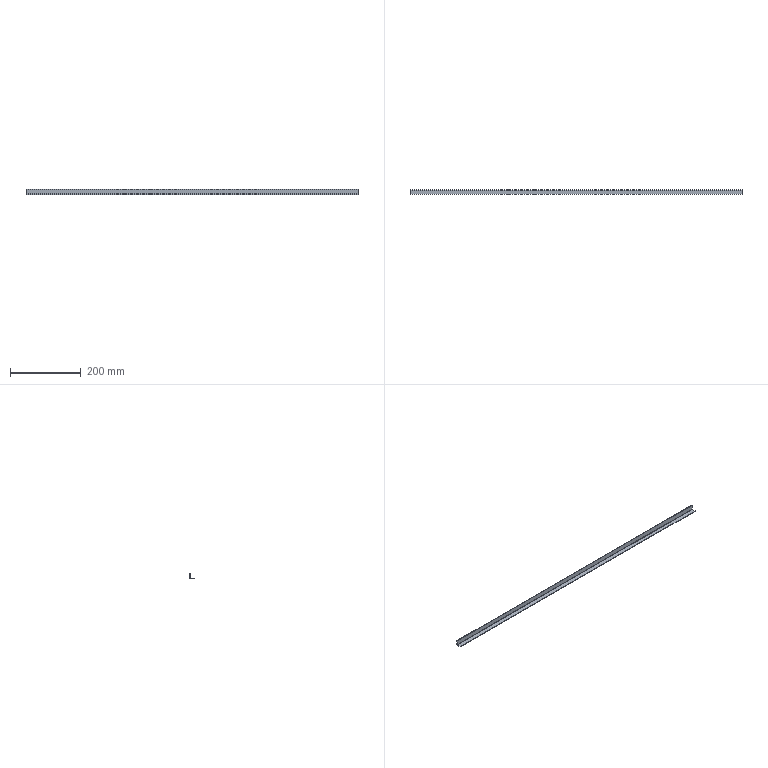Part | STEP file | Left Side Panel Frame Lower | 1 solid | 10 faces | box 940 x 13.5 x 15 mm | volume 37314 mm3 | plane 8 | cylinder 2 | commonest cylinder face diameters 1 x1 4 x1
STEP:
#1=CARTESIAN_POINT('',(940.,0.,0.));
#2=VERTEX_POINT('',#1);
#3=CARTESIAN_POINT('',(940.,0.,-13.));
#4=VERTEX_POINT('',#3);
#5=CARTESIAN_POINT('',(940.,0.,0.));
#6=DIRECTION('',(0.,0.,-1.));
#7=VECTOR('',#6,1000.);
#8=LINE('',#5,#7);
#9=EDGE_CURVE('',#2,#4,#8,.T.);
#10=ORIENTED_EDGE('',*,*,#9,.T.);
#11=CARTESIAN_POINT('',(0.,0.,-13.));
#12=VERTEX_POINT('',#11);
#13=CARTESIAN_POINT('',(940.,0.,-13.));
#14=DIRECTION('',(-1.,0.,0.));
#15=VECTOR('',#14,1000.);
#16=LINE('',#13,#15);
#17=EDGE_CURVE('',#4,#12,#16,.T.);
#18=ORIENTED_EDGE('',*,*,#17,.T.);
#19=CARTESIAN_POINT('',(0.,0.,0.));
#20=VERTEX_POINT('',#19);
#21=CARTESIAN_POINT('',(0.,0.,0.));
#22=DIRECTION('',(0.,0.,1.));
#23=VECTOR('',#22,1000.);
#24=LINE('',#21,#23);
#25=EDGE_CURVE('',#12,#20,#24,.T.);
#26=ORIENTED_EDGE('',*,*,#25,.T.);
#27=CARTESIAN_POINT('',(940.,0.,0.));
#28=DIRECTION('',(1.,0.,0.));
#29=VECTOR('',#28,1000.);
#30=LINE('',#27,#29);
#31=EDGE_CURVE('',#20,#2,#30,.T.);
#32=ORIENTED_EDGE('',*,*,#31,.T.);
#33=EDGE_LOOP('',(#10,#18,#26,#32));
#34=FACE_OUTER_BOUND('',#33,.T.);
#35=CARTESIAN_POINT('',(940.,0.,0.));
#36=DIRECTION('',(0.,1.,0.));
#37=DIRECTION('',(0.,0.,1.));
#38=AXIS2_PLACEMENT_3D('',#35,#36,#37);
#39=PLANE('',#38);
#40=ADVANCED_FACE('',(#34),#39,.T.);
#41=CARTESIAN_POINT('',(940.,-2.,-15.));
#42=VERTEX_POINT('',#41);
#43=CARTESIAN_POINT('',(940.,-2.,-13.));
#44=DIRECTION('',(-1.,0.,0.));
#45=DIRECTION('',(0.,0.,1.));
#46=AXIS2_PLACEMENT_3D('',#43,#44,#45);
#47=CIRCLE('',#46,2.);
#48=EDGE_CURVE('',#4,#42,#47,.T.);
#49=ORIENTED_EDGE('',*,*,#48,.T.);
#50=CARTESIAN_POINT('',(0.,-2.,-15.));
#51=VERTEX_POINT('',#50);
#52=CARTESIAN_POINT('',(940.,-2.,-15.));
#53=DIRECTION('',(-1.,0.,0.));
#54=VECTOR('',#53,1000.);
#55=LINE('',#52,#54);
#56=EDGE_CURVE('',#42,#51,#55,.T.);
#57=ORIENTED_EDGE('',*,*,#56,.T.);
#58=CARTESIAN_POINT('',(0.,-2.,-13.));
#59=DIRECTION('',(1.,0.,0.));
#60=DIRECTION('',(0.,0.,1.));
#61=AXIS2_PLACEMENT_3D('',#58,#59,#60);
#62=CIRCLE('',#61,2.);
#63=EDGE_CURVE('',#51,#12,#62,.T.);
#64=ORIENTED_EDGE('',*,*,#63,.T.);
#65=ORIENTED_EDGE('',*,*,#17,.F.);
#66=EDGE_LOOP('',(#49,#57,#64,#65));
#67=FACE_OUTER_BOUND('',#66,.T.);
#68=CARTESIAN_POINT('',(940.,-2.,-13.));
#69=DIRECTION('',(-1.,0.,0.));
#70=DIRECTION('',(0.,0.,1.));
#71=AXIS2_PLACEMENT_3D('',#68,#69,#70);
#72=CYLINDRICAL_SURFACE('',#71,2.);
#73=ADVANCED_FACE('',(#67),#72,.T.);
#74=ORIENTED_EDGE('',*,*,#9,.F.);
#75=CARTESIAN_POINT('',(940.,-1.5,0.));
#76=VERTEX_POINT('',#75);
#77=CARTESIAN_POINT('',(940.,-2.,0.));
#78=DIRECTION('',(0.,-1.,0.));
#79=VECTOR('',#78,1000.);
#80=LINE('',#77,#79);
#81=EDGE_CURVE('',#2,#76,#80,.T.);
#82=ORIENTED_EDGE('',*,*,#81,.T.);
#83=CARTESIAN_POINT('',(940.,-1.5,-13.));
#84=VERTEX_POINT('',#83);
#85=CARTESIAN_POINT('',(940.,-1.5,-13.));
#86=DIRECTION('',(0.,0.,-1.));
#87=VECTOR('',#86,1000.);
#88=LINE('',#85,#87);
#89=EDGE_CURVE('',#76,#84,#88,.T.);
#90=ORIENTED_EDGE('',*,*,#89,.T.);
#91=CARTESIAN_POINT('',(940.,-2.,-13.5));
#92=VERTEX_POINT('',#91);
#93=CARTESIAN_POINT('',(940.,-2.,-13.));
#94=DIRECTION('',(-1.,0.,0.));
#95=DIRECTION('',(0.,0.,1.));
#96=AXIS2_PLACEMENT_3D('',#93,#94,#95);
#97=CIRCLE('',#96,0.5);
#98=EDGE_CURVE('',#84,#92,#97,.T.);
#99=ORIENTED_EDGE('',*,*,#98,.T.);
#100=CARTESIAN_POINT('',(940.,-13.5,-13.5));
#101=VERTEX_POINT('',#100);
#102=CARTESIAN_POINT('',(940.,-1.5,-13.5));
#103=DIRECTION('',(0.,-1.,0.));
#104=VECTOR('',#103,1000.);
#105=LINE('',#102,#104);
#106=EDGE_CURVE('',#92,#101,#105,.T.);
#107=ORIENTED_EDGE('',*,*,#106,.T.);
#108=CARTESIAN_POINT('',(940.,-13.5,-15.));
#109=VERTEX_POINT('',#108);
#110=CARTESIAN_POINT('',(940.,-13.5,-15.));
#111=DIRECTION('',(0.,0.,1.));
#112=VECTOR('',#111,1000.);
#113=LINE('',#110,#112);
#114=EDGE_CURVE('',#109,#101,#113,.T.);
#115=ORIENTED_EDGE('',*,*,#114,.F.);
#116=CARTESIAN_POINT('',(940.,0.,-15.));
#117=DIRECTION('',(0.,-1.,0.));
#118=VECTOR('',#117,1000.);
#119=LINE('',#116,#118);
#120=EDGE_CURVE('',#42,#109,#119,.T.);
#121=ORIENTED_EDGE('',*,*,#120,.F.);
#122=ORIENTED_EDGE('',*,*,#48,.F.);
#123=EDGE_LOOP('',(#74,#82,#90,#99,#107,#115,#121,#122));
#124=FACE_OUTER_BOUND('',#123,.T.);
#125=CARTESIAN_POINT('',(940.,-2.,-13.));
#126=DIRECTION('',(1.,0.,0.));
#127=DIRECTION('',(0.,0.,-1.));
#128=AXIS2_PLACEMENT_3D('',#125,#126,#127);
#129=PLANE('',#128);
#130=ADVANCED_FACE('',(#124),#129,.T.);
#131=ORIENTED_EDGE('',*,*,#81,.F.);
#132=ORIENTED_EDGE('',*,*,#31,.F.);
#133=CARTESIAN_POINT('',(0.,-1.5,0.));
#134=VERTEX_POINT('',#133);
#135=CARTESIAN_POINT('',(0.,-1.5,0.));
#136=DIRECTION('',(0.,-1.,0.));
#137=VECTOR('',#136,1000.);
#138=LINE('',#135,#137);
#139=EDGE_CURVE('',#20,#134,#138,.T.);
#140=ORIENTED_EDGE('',*,*,#139,.T.);
#141=CARTESIAN_POINT('',(940.,-1.5,0.));
#142=DIRECTION('',(1.,0.,0.));
#143=VECTOR('',#142,1000.);
#144=LINE('',#141,#143);
#145=EDGE_CURVE('',#134,#76,#144,.T.);
#146=ORIENTED_EDGE('',*,*,#145,.T.);
#147=EDGE_LOOP('',(#131,#132,#140,#146));
#148=FACE_OUTER_BOUND('',#147,.T.);
#149=CARTESIAN_POINT('',(940.,-1.5,0.));
#150=DIRECTION('',(0.,0.,1.));
#151=DIRECTION('',(1.,0.,0.));
#152=AXIS2_PLACEMENT_3D('',#149,#150,#151);
#153=PLANE('',#152);
#154=ADVANCED_FACE('',(#148),#153,.T.);
#155=CARTESIAN_POINT('',(0.,-1.5,-13.));
#156=VERTEX_POINT('',#155);
#157=CARTESIAN_POINT('',(0.,-1.5,-13.5));
#158=DIRECTION('',(0.,0.,1.));
#159=VECTOR('',#158,1000.);
#160=LINE('',#157,#159);
#161=EDGE_CURVE('',#156,#134,#160,.T.);
#162=ORIENTED_EDGE('',*,*,#161,.T.);
#163=ORIENTED_EDGE('',*,*,#139,.F.);
#164=ORIENTED_EDGE('',*,*,#25,.F.);
#165=ORIENTED_EDGE('',*,*,#63,.F.);
#166=CARTESIAN_POINT('',(0.,-13.5,-15.));
#167=VERTEX_POINT('',#166);
#168=CARTESIAN_POINT('',(0.,0.,-15.));
#169=DIRECTION('',(0.,1.,0.));
#170=VECTOR('',#169,1000.);
#171=LINE('',#168,#170);
#172=EDGE_CURVE('',#167,#51,#171,.T.);
#173=ORIENTED_EDGE('',*,*,#172,.F.);
#174=CARTESIAN_POINT('',(0.,-13.5,-13.5));
#175=VERTEX_POINT('',#174);
#176=CARTESIAN_POINT('',(0.,-13.5,-15.));
#177=DIRECTION('',(0.,0.,-1.));
#178=VECTOR('',#177,1000.);
#179=LINE('',#176,#178);
#180=EDGE_CURVE('',#175,#167,#179,.T.);
#181=ORIENTED_EDGE('',*,*,#180,.F.);
#182=CARTESIAN_POINT('',(0.,-2.,-13.5));
#183=VERTEX_POINT('',#182);
#184=CARTESIAN_POINT('',(0.,-2.,-13.5));
#185=DIRECTION('',(0.,-1.,0.));
#186=VECTOR('',#185,1000.);
#187=LINE('',#184,#186);
#188=EDGE_CURVE('',#183,#175,#187,.T.);
#189=ORIENTED_EDGE('',*,*,#188,.F.);
#190=CARTESIAN_POINT('',(0.,-2.,-13.));
#191=DIRECTION('',(1.,0.,0.));
#192=DIRECTION('',(0.,0.,1.));
#193=AXIS2_PLACEMENT_3D('',#190,#191,#192);
#194=CIRCLE('',#193,0.5);
#195=EDGE_CURVE('',#183,#156,#194,.T.);
#196=ORIENTED_EDGE('',*,*,#195,.T.);
#197=EDGE_LOOP('',(#162,#163,#164,#165,#173,#181,#189,#196));
#198=FACE_OUTER_BOUND('',#197,.T.);
#199=CARTESIAN_POINT('',(0.,-2.,-13.5));
#200=DIRECTION('',(-1.,0.,0.));
#201=DIRECTION('',(0.,0.,1.));
#202=AXIS2_PLACEMENT_3D('',#199,#200,#201);
#203=PLANE('',#202);
#204=ADVANCED_FACE('',(#198),#203,.T.);
#205=ORIENTED_EDGE('',*,*,#120,.T.);
#206=CARTESIAN_POINT('',(940.,-13.5,-15.));
#207=DIRECTION('',(-1.,0.,0.));
#208=VECTOR('',#207,1000.);
#209=LINE('',#206,#208);
#210=EDGE_CURVE('',#109,#167,#209,.T.);
#211=ORIENTED_EDGE('',*,*,#210,.T.);
#212=ORIENTED_EDGE('',*,*,#172,.T.);
#213=ORIENTED_EDGE('',*,*,#56,.F.);
#214=EDGE_LOOP('',(#205,#211,#212,#213));
#215=FACE_OUTER_BOUND('',#214,.T.);
#216=CARTESIAN_POINT('',(940.,0.,-15.));
#217=DIRECTION('',(0.,0.,-1.));
#218=DIRECTION('',(0.,1.,0.));
#219=AXIS2_PLACEMENT_3D('',#216,#217,#218);
#220=PLANE('',#219);
#221=ADVANCED_FACE('',(#215),#220,.T.);
#222=CARTESIAN_POINT('',(940.,-1.5,-13.));
#223=DIRECTION('',(-1.,0.,0.));
#224=VECTOR('',#223,1000.);
#225=LINE('',#222,#224);
#226=EDGE_CURVE('',#84,#156,#225,.T.);
#227=ORIENTED_EDGE('',*,*,#226,.F.);
#228=ORIENTED_EDGE('',*,*,#89,.F.);
#229=ORIENTED_EDGE('',*,*,#145,.F.);
#230=ORIENTED_EDGE('',*,*,#161,.F.);
#231=EDGE_LOOP('',(#227,#228,#229,#230));
#232=FACE_OUTER_BOUND('',#231,.T.);
#233=CARTESIAN_POINT('',(940.,-1.5,0.));
#234=DIRECTION('',(0.,1.,0.));
#235=DIRECTION('',(0.,0.,1.));
#236=AXIS2_PLACEMENT_3D('',#233,#234,#235);
#237=PLANE('',#236);
#238=ADVANCED_FACE('',(#232),#237,.F.);
#239=ORIENTED_EDGE('',*,*,#114,.T.);
#240=CARTESIAN_POINT('',(940.,-13.5,-13.5));
#241=DIRECTION('',(-1.,0.,0.));
#242=VECTOR('',#241,1000.);
#243=LINE('',#240,#242);
#244=EDGE_CURVE('',#101,#175,#243,.T.);
#245=ORIENTED_EDGE('',*,*,#244,.T.);
#246=ORIENTED_EDGE('',*,*,#180,.T.);
#247=ORIENTED_EDGE('',*,*,#210,.F.);
#248=EDGE_LOOP('',(#239,#245,#246,#247));
#249=FACE_OUTER_BOUND('',#248,.T.);
#250=CARTESIAN_POINT('',(940.,-13.5,-15.));
#251=DIRECTION('',(0.,-1.,0.));
#252=DIRECTION('',(0.,0.,-1.));
#253=AXIS2_PLACEMENT_3D('',#250,#251,#252);
#254=PLANE('',#253);
#255=ADVANCED_FACE('',(#249),#254,.T.);
#256=CARTESIAN_POINT('',(940.,-2.,-13.5));
#257=DIRECTION('',(-1.,0.,0.));
#258=VECTOR('',#257,1000.);
#259=LINE('',#256,#258);
#260=EDGE_CURVE('',#92,#183,#259,.T.);
#261=ORIENTED_EDGE('',*,*,#260,.F.);
#262=ORIENTED_EDGE('',*,*,#98,.F.);
#263=ORIENTED_EDGE('',*,*,#226,.T.);
#264=ORIENTED_EDGE('',*,*,#195,.F.);
#265=EDGE_LOOP('',(#261,#262,#263,#264));
#266=FACE_OUTER_BOUND('',#265,.T.);
#267=CARTESIAN_POINT('',(940.,-2.,-13.));
#268=DIRECTION('',(-1.,0.,0.));
#269=DIRECTION('',(0.,0.,1.));
#270=AXIS2_PLACEMENT_3D('',#267,#268,#269);
#271=CYLINDRICAL_SURFACE('',#270,0.5);
#272=ADVANCED_FACE('',(#266),#271,.F.);
#273=ORIENTED_EDGE('',*,*,#244,.F.);
#274=ORIENTED_EDGE('',*,*,#106,.F.);
#275=ORIENTED_EDGE('',*,*,#260,.T.);
#276=ORIENTED_EDGE('',*,*,#188,.T.);
#277=EDGE_LOOP('',(#273,#274,#275,#276));
#278=FACE_OUTER_BOUND('',#277,.T.);
#279=CARTESIAN_POINT('',(940.,0.,-13.5));
#280=DIRECTION('',(0.,0.,-1.));
#281=DIRECTION('',(0.,1.,0.));
#282=AXIS2_PLACEMENT_3D('',#279,#280,#281);
#283=PLANE('',#282);
#284=ADVANCED_FACE('',(#278),#283,.F.);
#285=CLOSED_SHELL('',(#40,#73,#130,#154,#204,#221,#238,#255,#272,#284));
#286=MANIFOLD_SOLID_BREP('',#285);
#287=CARTESIAN_POINT('',(0.,0.,0.));
#288=DIRECTION('',(0.,0.,1.));
#289=DIRECTION('',(1.,0.,0.));
#290=AXIS2_PLACEMENT_3D('',#287,#288,#289);
#291=(LENGTH_UNIT()NAMED_UNIT(*)SI_UNIT(.MILLI.,.METRE.));
#292=UNCERTAINTY_MEASURE_WITH_UNIT(LENGTH_MEASURE(0.00001),#291,'','');
#293=(NAMED_UNIT(*)PLANE_ANGLE_UNIT()SI_UNIT($,.RADIAN.));
#294=(NAMED_UNIT(*)SI_UNIT($,.STERADIAN.)SOLID_ANGLE_UNIT());
#295=(GEOMETRIC_REPRESENTATION_CONTEXT(3)GLOBAL_UNCERTAINTY_ASSIGNED_CONTEXT((#292))GLOBAL_UNIT_ASSIGNED_CONTEXT((#291,#293,#294))REPRESENTATION_CONTEXT('',''));
#296=ADVANCED_BREP_SHAPE_REPRESENTATION('',(#286,#290),#295);